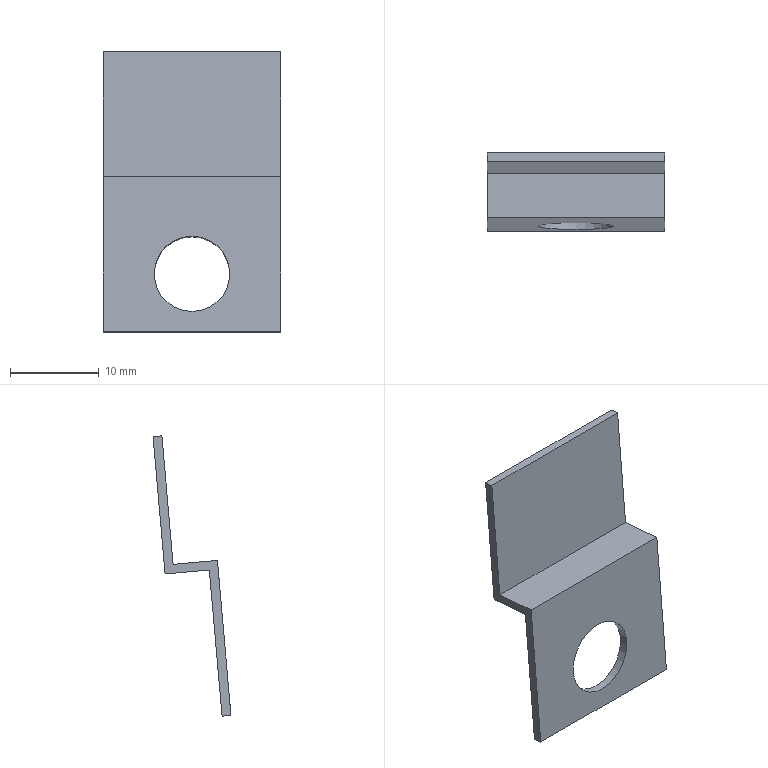Part | NX | features solid 2 | 1 solid | 11 faces | box 20 x 8.766 x 31.53 mm | volume 683.255 mm3 | plane 10 | cylinder 1 | commonest cylinder face diameters 8.5 x1
STEP:
#1=CARTESIAN_POINT('',(388.525,-119.54,-60.769));
#2=VERTEX_POINT('',#1);
#3=CARTESIAN_POINT('',(408.525,-119.54,-60.769));
#4=VERTEX_POINT('',#3);
#5=CARTESIAN_POINT('',(388.525,-119.54,-60.769));
#6=DIRECTION('',(1.,0.,0.));
#7=VECTOR('',#6,1000.);
#8=LINE('',#5,#7);
#9=EDGE_CURVE('',#2,#4,#8,.T.);
#10=ORIENTED_EDGE('',*,*,#9,.F.);
#11=CARTESIAN_POINT('',(388.525,-121.065,-78.202));
#12=VERTEX_POINT('',#11);
#13=CARTESIAN_POINT('',(388.525,-119.627,-61.765));
#14=DIRECTION('',(0.,0.08716,0.9962));
#15=VECTOR('',#14,1000.);
#16=LINE('',#13,#15);
#17=EDGE_CURVE('',#12,#2,#16,.T.);
#18=ORIENTED_EDGE('',*,*,#17,.F.);
#19=CARTESIAN_POINT('',(408.525,-121.065,-78.202));
#20=VERTEX_POINT('',#19);
#21=CARTESIAN_POINT('',(388.525,-121.065,-78.202));
#22=DIRECTION('',(1.,0.,0.));
#23=VECTOR('',#22,1000.);
#24=LINE('',#21,#23);
#25=EDGE_CURVE('',#12,#20,#24,.T.);
#26=ORIENTED_EDGE('',*,*,#25,.T.);
#27=CARTESIAN_POINT('',(408.525,-119.54,-60.769));
#28=DIRECTION('',(0.,-0.08716,-0.9962));
#29=VECTOR('',#28,1000.);
#30=LINE('',#27,#29);
#31=EDGE_CURVE('',#4,#20,#30,.T.);
#32=ORIENTED_EDGE('',*,*,#31,.F.);
#33=EDGE_LOOP('',(#10,#18,#26,#32));
#34=FACE_BOUND('',#33,.T.);
#35=CARTESIAN_POINT('',(398.525,-120.869,-75.961));
#36=VERTEX_POINT('',#35);
#37=CARTESIAN_POINT('',(398.525,-120.499,-71.727));
#38=DIRECTION('',(0.,0.9962,-0.08716));
#39=DIRECTION('',(0.,-0.08716,-0.9962));
#40=AXIS2_PLACEMENT_3D('',#37,#38,#39);
#41=CIRCLE('',#40,4.25);
#42=EDGE_CURVE('',#36,#36,#41,.T.);
#43=ORIENTED_EDGE('',*,*,#42,.T.);
#44=EDGE_LOOP('',(#43));
#45=FACE_BOUND('',#44,.T.);
#46=CARTESIAN_POINT('',(408.525,-119.54,-60.769));
#47=DIRECTION('',(0.,0.9962,-0.08716));
#48=DIRECTION('',(0.,-0.08716,-0.9962));
#49=AXIS2_PLACEMENT_3D('',#46,#47,#48);
#50=PLANE('',#49);
#51=ADVANCED_FACE('',(#34,#45),#50,.F.);
#52=CARTESIAN_POINT('',(388.525,-120.069,-78.29));
#53=VERTEX_POINT('',#52);
#54=CARTESIAN_POINT('',(408.525,-120.069,-78.29));
#55=VERTEX_POINT('',#54);
#56=CARTESIAN_POINT('',(388.525,-120.069,-78.29));
#57=DIRECTION('',(1.,0.,0.));
#58=VECTOR('',#57,1000.);
#59=LINE('',#56,#58);
#60=EDGE_CURVE('',#53,#55,#59,.T.);
#61=ORIENTED_EDGE('',*,*,#60,.F.);
#62=CARTESIAN_POINT('',(388.525,-118.631,-61.852));
#63=VERTEX_POINT('',#62);
#64=CARTESIAN_POINT('',(388.525,-118.631,-61.852));
#65=DIRECTION('',(0.,-0.08716,-0.9962));
#66=VECTOR('',#65,1000.);
#67=LINE('',#64,#66);
#68=EDGE_CURVE('',#63,#53,#67,.T.);
#69=ORIENTED_EDGE('',*,*,#68,.F.);
#70=CARTESIAN_POINT('',(408.525,-118.631,-61.852));
#71=VERTEX_POINT('',#70);
#72=CARTESIAN_POINT('',(388.525,-118.631,-61.852));
#73=DIRECTION('',(1.,0.,0.));
#74=VECTOR('',#73,1000.);
#75=LINE('',#72,#74);
#76=EDGE_CURVE('',#63,#71,#75,.T.);
#77=ORIENTED_EDGE('',*,*,#76,.T.);
#78=CARTESIAN_POINT('',(408.525,-120.069,-78.29));
#79=DIRECTION('',(0.,0.08716,0.9962));
#80=VECTOR('',#79,1000.);
#81=LINE('',#78,#80);
#82=EDGE_CURVE('',#55,#71,#81,.T.);
#83=ORIENTED_EDGE('',*,*,#82,.F.);
#84=EDGE_LOOP('',(#61,#69,#77,#83));
#85=FACE_BOUND('',#84,.T.);
#86=CARTESIAN_POINT('',(398.525,-119.873,-76.048));
#87=VERTEX_POINT('',#86);
#88=CARTESIAN_POINT('',(398.525,-119.503,-71.814));
#89=DIRECTION('',(0.,0.9962,-0.08716));
#90=DIRECTION('',(0.,-0.08716,-0.9962));
#91=AXIS2_PLACEMENT_3D('',#88,#89,#90);
#92=CIRCLE('',#91,4.25);
#93=EDGE_CURVE('',#87,#87,#92,.T.);
#94=ORIENTED_EDGE('',*,*,#93,.F.);
#95=EDGE_LOOP('',(#94));
#96=FACE_BOUND('',#95,.T.);
#97=CARTESIAN_POINT('',(408.525,-120.069,-78.29));
#98=DIRECTION('',(0.,-0.9962,0.08716));
#99=DIRECTION('',(0.,0.08716,0.9962));
#100=AXIS2_PLACEMENT_3D('',#97,#98,#99);
#101=PLANE('',#100);
#102=ADVANCED_FACE('',(#85,#96),#101,.F.);
#103=CARTESIAN_POINT('',(408.525,-113.295,-46.76));
#104=VERTEX_POINT('',#103);
#105=CARTESIAN_POINT('',(388.525,-113.295,-46.76));
#106=VERTEX_POINT('',#105);
#107=CARTESIAN_POINT('',(408.525,-113.295,-46.76));
#108=DIRECTION('',(-1.,0.,0.));
#109=VECTOR('',#108,1000.);
#110=LINE('',#107,#109);
#111=EDGE_CURVE('',#104,#106,#110,.T.);
#112=ORIENTED_EDGE('',*,*,#111,.F.);
#113=CARTESIAN_POINT('',(408.525,-112.299,-46.847));
#114=VERTEX_POINT('',#113);
#115=CARTESIAN_POINT('',(408.525,-112.299,-46.847));
#116=DIRECTION('',(0.,-0.9962,0.08716));
#117=VECTOR('',#116,1000.);
#118=LINE('',#115,#117);
#119=EDGE_CURVE('',#114,#104,#118,.T.);
#120=ORIENTED_EDGE('',*,*,#119,.F.);
#121=CARTESIAN_POINT('',(388.525,-112.299,-46.847));
#122=VERTEX_POINT('',#121);
#123=CARTESIAN_POINT('',(408.525,-112.299,-46.847));
#124=DIRECTION('',(-1.,0.,0.));
#125=VECTOR('',#124,1000.);
#126=LINE('',#123,#125);
#127=EDGE_CURVE('',#114,#122,#126,.T.);
#128=ORIENTED_EDGE('',*,*,#127,.T.);
#129=CARTESIAN_POINT('',(388.525,-112.299,-46.847));
#130=DIRECTION('',(0.,-0.9962,0.08716));
#131=VECTOR('',#130,1000.);
#132=LINE('',#129,#131);
#133=EDGE_CURVE('',#122,#106,#132,.T.);
#134=ORIENTED_EDGE('',*,*,#133,.T.);
#135=EDGE_LOOP('',(#112,#120,#128,#134));
#136=FACE_BOUND('',#135,.T.);
#137=CARTESIAN_POINT('',(408.525,-112.299,-46.847));
#138=DIRECTION('',(0.,0.08716,0.9962));
#139=DIRECTION('',(0.,0.9962,-0.08716));
#140=AXIS2_PLACEMENT_3D('',#137,#138,#139);
#141=PLANE('',#140);
#142=ADVANCED_FACE('',(#136),#141,.T.);
#143=CARTESIAN_POINT('',(388.525,-114.559,-61.205));
#144=VERTEX_POINT('',#143);
#145=CARTESIAN_POINT('',(388.525,-113.295,-46.76));
#146=DIRECTION('',(0.,-0.08716,-0.9962));
#147=VECTOR('',#146,1000.);
#148=LINE('',#145,#147);
#149=EDGE_CURVE('',#106,#144,#148,.T.);
#150=ORIENTED_EDGE('',*,*,#149,.F.);
#151=ORIENTED_EDGE('',*,*,#133,.F.);
#152=CARTESIAN_POINT('',(388.525,-113.65,-62.288));
#153=VERTEX_POINT('',#152);
#154=CARTESIAN_POINT('',(388.525,-112.299,-46.847));
#155=DIRECTION('',(0.,-0.08716,-0.9962));
#156=VECTOR('',#155,1000.);
#157=LINE('',#154,#156);
#158=EDGE_CURVE('',#122,#153,#157,.T.);
#159=ORIENTED_EDGE('',*,*,#158,.T.);
#160=CARTESIAN_POINT('',(388.525,-113.65,-62.288));
#161=DIRECTION('',(0.,-0.9962,0.08716));
#162=VECTOR('',#161,1000.);
#163=LINE('',#160,#162);
#164=EDGE_CURVE('',#153,#63,#163,.T.);
#165=ORIENTED_EDGE('',*,*,#164,.T.);
#166=ORIENTED_EDGE('',*,*,#68,.T.);
#167=CARTESIAN_POINT('',(388.525,-120.069,-78.29));
#168=DIRECTION('',(0.,-0.9962,0.08716));
#169=VECTOR('',#168,1000.);
#170=LINE('',#167,#169);
#171=EDGE_CURVE('',#53,#12,#170,.T.);
#172=ORIENTED_EDGE('',*,*,#171,.T.);
#173=ORIENTED_EDGE('',*,*,#17,.T.);
#174=CARTESIAN_POINT('',(388.525,-113.563,-61.292));
#175=DIRECTION('',(0.,-0.9962,0.08716));
#176=VECTOR('',#175,1000.);
#177=LINE('',#174,#176);
#178=EDGE_CURVE('',#144,#2,#177,.T.);
#179=ORIENTED_EDGE('',*,*,#178,.F.);
#180=EDGE_LOOP('',(#150,#151,#159,#165,#166,#172,#173,#179));
#181=FACE_BOUND('',#180,.T.);
#182=CARTESIAN_POINT('',(388.525,-112.299,-46.847));
#183=DIRECTION('',(-1.,0.,0.));
#184=DIRECTION('',(0.,0.9962,-0.08716));
#185=AXIS2_PLACEMENT_3D('',#182,#183,#184);
#186=PLANE('',#185);
#187=ADVANCED_FACE('',(#181),#186,.T.);
#188=CARTESIAN_POINT('',(408.525,-114.559,-61.205));
#189=VERTEX_POINT('',#188);
#190=CARTESIAN_POINT('',(408.525,-114.559,-61.205));
#191=DIRECTION('',(0.,0.08716,0.9962));
#192=VECTOR('',#191,1000.);
#193=LINE('',#190,#192);
#194=EDGE_CURVE('',#189,#104,#193,.T.);
#195=ORIENTED_EDGE('',*,*,#194,.F.);
#196=CARTESIAN_POINT('',(408.525,-113.563,-61.292));
#197=DIRECTION('',(0.,-0.9962,0.08716));
#198=VECTOR('',#197,1000.);
#199=LINE('',#196,#198);
#200=EDGE_CURVE('',#189,#4,#199,.T.);
#201=ORIENTED_EDGE('',*,*,#200,.T.);
#202=ORIENTED_EDGE('',*,*,#31,.T.);
#203=CARTESIAN_POINT('',(408.525,-120.069,-78.29));
#204=DIRECTION('',(0.,-0.9962,0.08716));
#205=VECTOR('',#204,1000.);
#206=LINE('',#203,#205);
#207=EDGE_CURVE('',#55,#20,#206,.T.);
#208=ORIENTED_EDGE('',*,*,#207,.F.);
#209=ORIENTED_EDGE('',*,*,#82,.T.);
#210=CARTESIAN_POINT('',(408.525,-113.65,-62.288));
#211=VERTEX_POINT('',#210);
#212=CARTESIAN_POINT('',(408.525,-113.65,-62.288));
#213=DIRECTION('',(0.,-0.9962,0.08716));
#214=VECTOR('',#213,1000.);
#215=LINE('',#212,#214);
#216=EDGE_CURVE('',#211,#71,#215,.T.);
#217=ORIENTED_EDGE('',*,*,#216,.F.);
#218=CARTESIAN_POINT('',(408.525,-113.563,-61.292));
#219=DIRECTION('',(0.,0.08716,0.9962));
#220=VECTOR('',#219,1000.);
#221=LINE('',#218,#220);
#222=EDGE_CURVE('',#211,#114,#221,.T.);
#223=ORIENTED_EDGE('',*,*,#222,.T.);
#224=ORIENTED_EDGE('',*,*,#119,.T.);
#225=EDGE_LOOP('',(#195,#201,#202,#208,#209,#217,#223,#224));
#226=FACE_BOUND('',#225,.T.);
#227=CARTESIAN_POINT('',(408.525,-113.563,-61.292));
#228=DIRECTION('',(1.,0.,0.));
#229=DIRECTION('',(0.,-0.08716,-0.9962));
#230=AXIS2_PLACEMENT_3D('',#227,#228,#229);
#231=PLANE('',#230);
#232=ADVANCED_FACE('',(#226),#231,.T.);
#233=ORIENTED_EDGE('',*,*,#127,.F.);
#234=ORIENTED_EDGE('',*,*,#222,.F.);
#235=CARTESIAN_POINT('',(388.525,-113.65,-62.288));
#236=DIRECTION('',(1.,0.,0.));
#237=VECTOR('',#236,1000.);
#238=LINE('',#235,#237);
#239=EDGE_CURVE('',#153,#211,#238,.T.);
#240=ORIENTED_EDGE('',*,*,#239,.F.);
#241=ORIENTED_EDGE('',*,*,#158,.F.);
#242=EDGE_LOOP('',(#233,#234,#240,#241));
#243=FACE_BOUND('',#242,.T.);
#244=CARTESIAN_POINT('',(388.525,-112.299,-46.847));
#245=DIRECTION('',(0.,-0.9962,0.08716));
#246=DIRECTION('',(0.,0.08716,0.9962));
#247=AXIS2_PLACEMENT_3D('',#244,#245,#246);
#248=PLANE('',#247);
#249=ADVANCED_FACE('',(#243),#248,.F.);
#250=ORIENTED_EDGE('',*,*,#111,.T.);
#251=ORIENTED_EDGE('',*,*,#149,.T.);
#252=CARTESIAN_POINT('',(388.525,-114.559,-61.205));
#253=DIRECTION('',(1.,0.,0.));
#254=VECTOR('',#253,1000.);
#255=LINE('',#252,#254);
#256=EDGE_CURVE('',#144,#189,#255,.T.);
#257=ORIENTED_EDGE('',*,*,#256,.T.);
#258=ORIENTED_EDGE('',*,*,#194,.T.);
#259=EDGE_LOOP('',(#250,#251,#257,#258));
#260=FACE_BOUND('',#259,.T.);
#261=CARTESIAN_POINT('',(388.525,-113.295,-46.76));
#262=DIRECTION('',(0.,-0.9962,0.08716));
#263=DIRECTION('',(0.,0.08716,0.9962));
#264=AXIS2_PLACEMENT_3D('',#261,#262,#263);
#265=PLANE('',#264);
#266=ADVANCED_FACE('',(#260),#265,.T.);
#267=ORIENTED_EDGE('',*,*,#256,.F.);
#268=ORIENTED_EDGE('',*,*,#178,.T.);
#269=ORIENTED_EDGE('',*,*,#9,.T.);
#270=ORIENTED_EDGE('',*,*,#200,.F.);
#271=EDGE_LOOP('',(#267,#268,#269,#270));
#272=FACE_BOUND('',#271,.T.);
#273=CARTESIAN_POINT('',(388.525,-113.563,-61.292));
#274=DIRECTION('',(0.,-0.08716,-0.9962));
#275=DIRECTION('',(0.,-0.9962,0.08716));
#276=AXIS2_PLACEMENT_3D('',#273,#274,#275);
#277=PLANE('',#276);
#278=ADVANCED_FACE('',(#272),#277,.F.);
#279=ORIENTED_EDGE('',*,*,#76,.F.);
#280=ORIENTED_EDGE('',*,*,#164,.F.);
#281=ORIENTED_EDGE('',*,*,#239,.T.);
#282=ORIENTED_EDGE('',*,*,#216,.T.);
#283=EDGE_LOOP('',(#279,#280,#281,#282));
#284=FACE_BOUND('',#283,.T.);
#285=CARTESIAN_POINT('',(388.525,-113.65,-62.288));
#286=DIRECTION('',(0.,-0.08716,-0.9962));
#287=DIRECTION('',(0.,-0.9962,0.08716));
#288=AXIS2_PLACEMENT_3D('',#285,#286,#287);
#289=PLANE('',#288);
#290=ADVANCED_FACE('',(#284),#289,.T.);
#291=ORIENTED_EDGE('',*,*,#25,.F.);
#292=ORIENTED_EDGE('',*,*,#171,.F.);
#293=ORIENTED_EDGE('',*,*,#60,.T.);
#294=ORIENTED_EDGE('',*,*,#207,.T.);
#295=EDGE_LOOP('',(#291,#292,#293,#294));
#296=FACE_BOUND('',#295,.T.);
#297=CARTESIAN_POINT('',(388.525,-120.069,-78.29));
#298=DIRECTION('',(0.,-0.08716,-0.9962));
#299=DIRECTION('',(0.,-0.9962,0.08716));
#300=AXIS2_PLACEMENT_3D('',#297,#298,#299);
#301=PLANE('',#300);
#302=ADVANCED_FACE('',(#296),#301,.T.);
#303=ORIENTED_EDGE('',*,*,#93,.T.);
#304=EDGE_LOOP('',(#303));
#305=FACE_BOUND('',#304,.T.);
#306=ORIENTED_EDGE('',*,*,#42,.F.);
#307=EDGE_LOOP('',(#306));
#308=FACE_BOUND('',#307,.T.);
#309=CARTESIAN_POINT('',(398.525,-119.503,-71.814));
#310=DIRECTION('',(0.,-0.9962,0.08716));
#311=DIRECTION('',(0.,0.08716,0.9962));
#312=AXIS2_PLACEMENT_3D('',#309,#310,#311);
#313=CYLINDRICAL_SURFACE('',#312,4.25);
#314=ADVANCED_FACE('',(#305,#308),#313,.F.);
#315=CLOSED_SHELL('',(#51,#102,#142,#187,#232,#249,#266,#278,#290,#302,#314));
#316=MANIFOLD_SOLID_BREP('',#315);
#317=(LENGTH_UNIT()NAMED_UNIT(*)SI_UNIT(.MILLI.,.METRE.));
#318=UNCERTAINTY_MEASURE_WITH_UNIT(LENGTH_MEASURE(0.00001),#317,'','');
#319=(NAMED_UNIT(*)PLANE_ANGLE_UNIT()SI_UNIT($,.RADIAN.));
#320=(NAMED_UNIT(*)SI_UNIT($,.STERADIAN.)SOLID_ANGLE_UNIT());
#321=(GEOMETRIC_REPRESENTATION_CONTEXT(3)GLOBAL_UNCERTAINTY_ASSIGNED_CONTEXT((#318))GLOBAL_UNIT_ASSIGNED_CONTEXT((#317,#319,#320))REPRESENTATION_CONTEXT('',''));
#322=ADVANCED_BREP_SHAPE_REPRESENTATION('',(#316),#321);